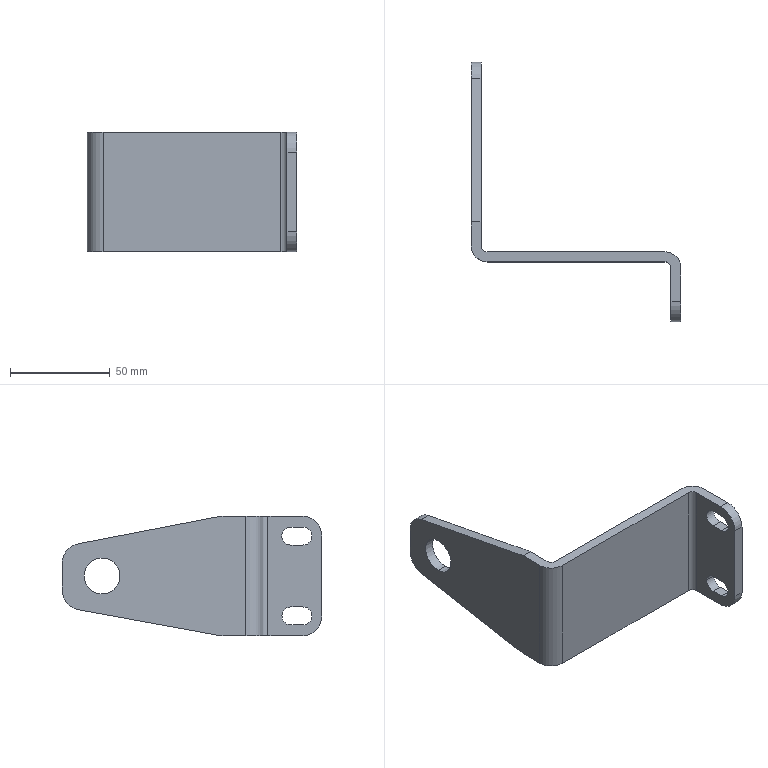Part | SolidWorks | features ICE 4, Fillet 3, Extrusion 1, HoleWzd 1 | 1 solid | 31 faces | box 105 x 130 x 60 mm | volume 58783 mm3 | plane 16 | cylinder 15 | commonest cylinder face diameters 9 x5 20 x4 6 x2 16 x2 18 x2
STEP:
#1=CARTESIAN_POINT('',(0.,-20.,39.));
#2=VERTEX_POINT('',#1);
#3=CARTESIAN_POINT('',(0.,-20.,21.));
#4=VERTEX_POINT('',#3);
#5=CARTESIAN_POINT('',(0.,-20.,30.));
#6=DIRECTION('',(1.,0.,0.));
#7=DIRECTION('',(0.,0.,-1.));
#8=AXIS2_PLACEMENT_3D('',#5,#6,#7);
#9=CIRCLE('',#8,9.);
#10=EDGE_CURVE('',#2,#4,#9,.T.);
#11=ORIENTED_EDGE('',*,*,#10,.T.);
#12=CARTESIAN_POINT('',(-5.,-20.,21.));
#13=VERTEX_POINT('',#12);
#14=CARTESIAN_POINT('',(-5.,-20.,21.));
#15=DIRECTION('',(-1.,0.,0.));
#16=VECTOR('',#15,1000.);
#17=LINE('',#14,#16);
#18=EDGE_CURVE('',#4,#13,#17,.T.);
#19=ORIENTED_EDGE('',*,*,#18,.T.);
#20=CARTESIAN_POINT('',(-5.,-20.,39.));
#21=VERTEX_POINT('',#20);
#22=CARTESIAN_POINT('',(-5.,-20.,30.));
#23=DIRECTION('',(-1.,0.,0.));
#24=DIRECTION('',(0.,0.,1.));
#25=AXIS2_PLACEMENT_3D('',#22,#23,#24);
#26=CIRCLE('',#25,9.);
#27=EDGE_CURVE('',#13,#21,#26,.T.);
#28=ORIENTED_EDGE('',*,*,#27,.T.);
#29=CARTESIAN_POINT('',(-5.,-20.,39.));
#30=DIRECTION('',(-1.,0.,0.));
#31=VECTOR('',#30,1000.);
#32=LINE('',#29,#31);
#33=EDGE_CURVE('',#2,#21,#32,.T.);
#34=ORIENTED_EDGE('',*,*,#33,.F.);
#35=EDGE_LOOP('',(#11,#19,#28,#34));
#36=FACE_OUTER_BOUND('',#35,.T.);
#37=CARTESIAN_POINT('',(-5.,-20.,30.));
#38=DIRECTION('',(-1.,0.,0.));
#39=DIRECTION('',(0.,0.,1.));
#40=AXIS2_PLACEMENT_3D('',#37,#38,#39);
#41=CYLINDRICAL_SURFACE('',#40,9.);
#42=ADVANCED_FACE('',(#36),#41,.F.);
#43=CARTESIAN_POINT('',(95.,-110.,10.));
#44=VERTEX_POINT('',#43);
#45=CARTESIAN_POINT('',(95.,-114.5,14.5));
#46=VERTEX_POINT('',#45);
#47=CARTESIAN_POINT('',(95.,-114.5,10.));
#48=DIRECTION('',(1.,0.,0.));
#49=DIRECTION('',(0.,0.,-1.));
#50=AXIS2_PLACEMENT_3D('',#47,#48,#49);
#51=CIRCLE('',#50,4.5);
#52=EDGE_CURVE('',#44,#46,#51,.T.);
#53=ORIENTED_EDGE('',*,*,#52,.F.);
#54=CARTESIAN_POINT('',(100.,-110.,10.));
#55=VERTEX_POINT('',#54);
#56=CARTESIAN_POINT('',(-5.,-110.,10.));
#57=DIRECTION('',(1.,0.,0.));
#58=VECTOR('',#57,1000.);
#59=LINE('',#56,#58);
#60=EDGE_CURVE('',#44,#55,#59,.T.);
#61=ORIENTED_EDGE('',*,*,#60,.T.);
#62=CARTESIAN_POINT('',(100.,-114.5,14.5));
#63=VERTEX_POINT('',#62);
#64=CARTESIAN_POINT('',(100.,-114.5,10.));
#65=DIRECTION('',(1.,0.,0.));
#66=DIRECTION('',(0.,1.,0.));
#67=AXIS2_PLACEMENT_3D('',#64,#65,#66);
#68=CIRCLE('',#67,4.5);
#69=EDGE_CURVE('',#55,#63,#68,.T.);
#70=ORIENTED_EDGE('',*,*,#69,.T.);
#71=CARTESIAN_POINT('',(-5.,-114.5,14.5));
#72=DIRECTION('',(1.,0.,0.));
#73=VECTOR('',#72,1000.);
#74=LINE('',#71,#73);
#75=EDGE_CURVE('',#46,#63,#74,.T.);
#76=ORIENTED_EDGE('',*,*,#75,.F.);
#77=EDGE_LOOP('',(#53,#61,#70,#76));
#78=FACE_OUTER_BOUND('',#77,.T.);
#79=CARTESIAN_POINT('',(-5.,-114.5,10.));
#80=DIRECTION('',(1.,0.,0.));
#81=DIRECTION('',(0.,1.,0.));
#82=AXIS2_PLACEMENT_3D('',#79,#80,#81);
#83=CYLINDRICAL_SURFACE('',#82,4.5);
#84=ADVANCED_FACE('',(#78),#83,.F.);
#85=CARTESIAN_POINT('',(100.,-120.,0.));
#86=VERTEX_POINT('',#85);
#87=CARTESIAN_POINT('',(100.,-103.,0.));
#88=VERTEX_POINT('',#87);
#89=CARTESIAN_POINT('',(100.,-95.,0.));
#90=DIRECTION('',(0.,1.,0.));
#91=VECTOR('',#90,1000.);
#92=LINE('',#89,#91);
#93=EDGE_CURVE('',#86,#88,#92,.T.);
#94=ORIENTED_EDGE('',*,*,#93,.F.);
#95=CARTESIAN_POINT('',(95.,-120.,0.));
#96=VERTEX_POINT('',#95);
#97=CARTESIAN_POINT('',(-5.,-120.,0.));
#98=DIRECTION('',(-1.,0.,0.));
#99=VECTOR('',#98,1000.);
#100=LINE('',#97,#99);
#101=EDGE_CURVE('',#86,#96,#100,.T.);
#102=ORIENTED_EDGE('',*,*,#101,.T.);
#103=CARTESIAN_POINT('',(95.,-103.,0.));
#104=VERTEX_POINT('',#103);
#105=CARTESIAN_POINT('',(95.,-100.,0.));
#106=DIRECTION('',(0.,-1.,0.));
#107=VECTOR('',#106,1000.);
#108=LINE('',#105,#107);
#109=EDGE_CURVE('',#104,#96,#108,.T.);
#110=ORIENTED_EDGE('',*,*,#109,.F.);
#111=CARTESIAN_POINT('',(92.,-100.,0.));
#112=VERTEX_POINT('',#111);
#113=CARTESIAN_POINT('',(92.,-103.,0.));
#114=DIRECTION('',(0.,0.,1.));
#115=DIRECTION('',(-1.,0.,0.));
#116=AXIS2_PLACEMENT_3D('',#113,#114,#115);
#117=CIRCLE('',#116,3.);
#118=EDGE_CURVE('',#104,#112,#117,.T.);
#119=ORIENTED_EDGE('',*,*,#118,.T.);
#120=CARTESIAN_POINT('',(3.,-100.,0.));
#121=VERTEX_POINT('',#120);
#122=CARTESIAN_POINT('',(-5.,-100.,0.));
#123=DIRECTION('',(1.,0.,0.));
#124=VECTOR('',#123,1000.);
#125=LINE('',#122,#124);
#126=EDGE_CURVE('',#121,#112,#125,.T.);
#127=ORIENTED_EDGE('',*,*,#126,.F.);
#128=CARTESIAN_POINT('',(-5.,-92.,0.));
#129=VERTEX_POINT('',#128);
#130=CARTESIAN_POINT('',(3.,-92.,0.));
#131=DIRECTION('',(0.,0.,-1.));
#132=DIRECTION('',(-1.,0.,0.));
#133=AXIS2_PLACEMENT_3D('',#130,#131,#132);
#134=CIRCLE('',#133,8.);
#135=EDGE_CURVE('',#121,#129,#134,.T.);
#136=ORIENTED_EDGE('',*,*,#135,.T.);
#137=CARTESIAN_POINT('',(-5.,-80.,0.));
#138=VERTEX_POINT('',#137);
#139=CARTESIAN_POINT('',(-5.,-130.,0.));
#140=DIRECTION('',(0.,1.,0.));
#141=VECTOR('',#140,1000.);
#142=LINE('',#139,#141);
#143=EDGE_CURVE('',#129,#138,#142,.T.);
#144=ORIENTED_EDGE('',*,*,#143,.T.);
#145=CARTESIAN_POINT('',(0.,-80.,0.));
#146=VERTEX_POINT('',#145);
#147=CARTESIAN_POINT('',(-5.,-80.,0.));
#148=DIRECTION('',(1.,0.,0.));
#149=VECTOR('',#148,1000.);
#150=LINE('',#147,#149);
#151=EDGE_CURVE('',#138,#146,#150,.T.);
#152=ORIENTED_EDGE('',*,*,#151,.T.);
#153=CARTESIAN_POINT('',(0.,-92.,0.));
#154=VERTEX_POINT('',#153);
#155=CARTESIAN_POINT('',(0.,-130.,0.));
#156=DIRECTION('',(0.,1.,0.));
#157=VECTOR('',#156,1000.);
#158=LINE('',#155,#157);
#159=EDGE_CURVE('',#154,#146,#158,.T.);
#160=ORIENTED_EDGE('',*,*,#159,.F.);
#161=CARTESIAN_POINT('',(3.,-95.,0.));
#162=VERTEX_POINT('',#161);
#163=CARTESIAN_POINT('',(3.,-92.,0.));
#164=DIRECTION('',(0.,0.,1.));
#165=DIRECTION('',(-1.,0.,0.));
#166=AXIS2_PLACEMENT_3D('',#163,#164,#165);
#167=CIRCLE('',#166,3.);
#168=EDGE_CURVE('',#154,#162,#167,.T.);
#169=ORIENTED_EDGE('',*,*,#168,.T.);
#170=CARTESIAN_POINT('',(92.,-95.,0.));
#171=VERTEX_POINT('',#170);
#172=CARTESIAN_POINT('',(100.,-95.,0.));
#173=DIRECTION('',(-1.,0.,0.));
#174=VECTOR('',#173,1000.);
#175=LINE('',#172,#174);
#176=EDGE_CURVE('',#171,#162,#175,.T.);
#177=ORIENTED_EDGE('',*,*,#176,.F.);
#178=CARTESIAN_POINT('',(92.,-103.,0.));
#179=DIRECTION('',(0.,0.,-1.));
#180=DIRECTION('',(-1.,0.,0.));
#181=AXIS2_PLACEMENT_3D('',#178,#179,#180);
#182=CIRCLE('',#181,8.);
#183=EDGE_CURVE('',#171,#88,#182,.T.);
#184=ORIENTED_EDGE('',*,*,#183,.T.);
#185=EDGE_LOOP('',(#94,#102,#110,#119,#127,#136,#144,#152,#160,#169,#177,#184));
#186=FACE_OUTER_BOUND('',#185,.T.);
#187=CARTESIAN_POINT('',(-5.,-130.,0.));
#188=DIRECTION('',(0.,0.,-1.));
#189=DIRECTION('',(-1.,0.,0.));
#190=AXIS2_PLACEMENT_3D('',#187,#188,#189);
#191=PLANE('',#190);
#192=ADVANCED_FACE('',(#186),#191,.T.);
#193=CARTESIAN_POINT('',(100.,-130.,50.));
#194=VERTEX_POINT('',#193);
#195=CARTESIAN_POINT('',(100.,-130.,10.));
#196=VERTEX_POINT('',#195);
#197=CARTESIAN_POINT('',(100.,-130.,0.));
#198=DIRECTION('',(0.,0.,-1.));
#199=VECTOR('',#198,1000.);
#200=LINE('',#197,#199);
#201=EDGE_CURVE('',#194,#196,#200,.T.);
#202=ORIENTED_EDGE('',*,*,#201,.F.);
#203=CARTESIAN_POINT('',(95.,-130.,50.));
#204=VERTEX_POINT('',#203);
#205=CARTESIAN_POINT('',(-5.,-130.,50.));
#206=DIRECTION('',(-1.,0.,0.));
#207=VECTOR('',#206,1000.);
#208=LINE('',#205,#207);
#209=EDGE_CURVE('',#194,#204,#208,.T.);
#210=ORIENTED_EDGE('',*,*,#209,.T.);
#211=CARTESIAN_POINT('',(95.,-130.,10.));
#212=VERTEX_POINT('',#211);
#213=CARTESIAN_POINT('',(95.,-130.,60.));
#214=DIRECTION('',(0.,0.,-1.));
#215=VECTOR('',#214,1000.);
#216=LINE('',#213,#215);
#217=EDGE_CURVE('',#204,#212,#216,.T.);
#218=ORIENTED_EDGE('',*,*,#217,.T.);
#219=CARTESIAN_POINT('',(-5.,-130.,10.));
#220=DIRECTION('',(1.,0.,0.));
#221=VECTOR('',#220,1000.);
#222=LINE('',#219,#221);
#223=EDGE_CURVE('',#212,#196,#222,.T.);
#224=ORIENTED_EDGE('',*,*,#223,.T.);
#225=EDGE_LOOP('',(#202,#210,#218,#224));
#226=FACE_OUTER_BOUND('',#225,.T.);
#227=CARTESIAN_POINT('',(-5.,-130.,60.));
#228=DIRECTION('',(0.,-1.,0.));
#229=DIRECTION('',(0.,0.,-1.));
#230=AXIS2_PLACEMENT_3D('',#227,#228,#229);
#231=PLANE('',#230);
#232=ADVANCED_FACE('',(#226),#231,.T.);
#233=CARTESIAN_POINT('',(95.,-103.,60.));
#234=VERTEX_POINT('',#233);
#235=CARTESIAN_POINT('',(95.,-120.,60.));
#236=VERTEX_POINT('',#235);
#237=CARTESIAN_POINT('',(95.,-100.,60.));
#238=DIRECTION('',(0.,-1.,0.));
#239=VECTOR('',#238,1000.);
#240=LINE('',#237,#239);
#241=EDGE_CURVE('',#234,#236,#240,.T.);
#242=ORIENTED_EDGE('',*,*,#241,.T.);
#243=CARTESIAN_POINT('',(100.,-120.,60.));
#244=VERTEX_POINT('',#243);
#245=CARTESIAN_POINT('',(-5.,-120.,60.));
#246=DIRECTION('',(1.,0.,0.));
#247=VECTOR('',#246,1000.);
#248=LINE('',#245,#247);
#249=EDGE_CURVE('',#236,#244,#248,.T.);
#250=ORIENTED_EDGE('',*,*,#249,.T.);
#251=CARTESIAN_POINT('',(100.,-103.,60.));
#252=VERTEX_POINT('',#251);
#253=CARTESIAN_POINT('',(100.,-130.,60.));
#254=DIRECTION('',(0.,-1.,0.));
#255=VECTOR('',#254,1000.);
#256=LINE('',#253,#255);
#257=EDGE_CURVE('',#252,#244,#256,.T.);
#258=ORIENTED_EDGE('',*,*,#257,.F.);
#259=CARTESIAN_POINT('',(92.,-95.,60.));
#260=VERTEX_POINT('',#259);
#261=CARTESIAN_POINT('',(92.,-103.,60.));
#262=DIRECTION('',(0.,0.,1.));
#263=DIRECTION('',(1.,0.,0.));
#264=AXIS2_PLACEMENT_3D('',#261,#262,#263);
#265=CIRCLE('',#264,8.);
#266=EDGE_CURVE('',#252,#260,#265,.T.);
#267=ORIENTED_EDGE('',*,*,#266,.T.);
#268=CARTESIAN_POINT('',(3.,-95.,60.));
#269=VERTEX_POINT('',#268);
#270=CARTESIAN_POINT('',(100.,-95.,60.));
#271=DIRECTION('',(-1.,0.,0.));
#272=VECTOR('',#271,1000.);
#273=LINE('',#270,#272);
#274=EDGE_CURVE('',#260,#269,#273,.T.);
#275=ORIENTED_EDGE('',*,*,#274,.T.);
#276=CARTESIAN_POINT('',(0.,-92.,60.));
#277=VERTEX_POINT('',#276);
#278=CARTESIAN_POINT('',(3.,-92.,60.));
#279=DIRECTION('',(0.,0.,-1.));
#280=DIRECTION('',(1.,0.,0.));
#281=AXIS2_PLACEMENT_3D('',#278,#279,#280);
#282=CIRCLE('',#281,3.);
#283=EDGE_CURVE('',#269,#277,#282,.T.);
#284=ORIENTED_EDGE('',*,*,#283,.T.);
#285=CARTESIAN_POINT('',(0.,-80.,60.));
#286=VERTEX_POINT('',#285);
#287=CARTESIAN_POINT('',(0.,-80.,60.));
#288=DIRECTION('',(0.,-1.,0.));
#289=VECTOR('',#288,1000.);
#290=LINE('',#287,#289);
#291=EDGE_CURVE('',#286,#277,#290,.T.);
#292=ORIENTED_EDGE('',*,*,#291,.F.);
#293=CARTESIAN_POINT('',(-5.,-80.,60.));
#294=VERTEX_POINT('',#293);
#295=CARTESIAN_POINT('',(-5.,-80.,60.));
#296=DIRECTION('',(1.,0.,0.));
#297=VECTOR('',#296,1000.);
#298=LINE('',#295,#297);
#299=EDGE_CURVE('',#294,#286,#298,.T.);
#300=ORIENTED_EDGE('',*,*,#299,.F.);
#301=CARTESIAN_POINT('',(-5.,-92.,60.));
#302=VERTEX_POINT('',#301);
#303=CARTESIAN_POINT('',(-5.,-80.,60.));
#304=DIRECTION('',(0.,-1.,0.));
#305=VECTOR('',#304,1000.);
#306=LINE('',#303,#305);
#307=EDGE_CURVE('',#294,#302,#306,.T.);
#308=ORIENTED_EDGE('',*,*,#307,.T.);
#309=CARTESIAN_POINT('',(3.,-100.,60.));
#310=VERTEX_POINT('',#309);
#311=CARTESIAN_POINT('',(3.,-92.,60.));
#312=DIRECTION('',(0.,0.,1.));
#313=DIRECTION('',(1.,0.,0.));
#314=AXIS2_PLACEMENT_3D('',#311,#312,#313);
#315=CIRCLE('',#314,8.);
#316=EDGE_CURVE('',#302,#310,#315,.T.);
#317=ORIENTED_EDGE('',*,*,#316,.T.);
#318=CARTESIAN_POINT('',(92.,-100.,60.));
#319=VERTEX_POINT('',#318);
#320=CARTESIAN_POINT('',(-5.,-100.,60.));
#321=DIRECTION('',(1.,0.,0.));
#322=VECTOR('',#321,1000.);
#323=LINE('',#320,#322);
#324=EDGE_CURVE('',#310,#319,#323,.T.);
#325=ORIENTED_EDGE('',*,*,#324,.T.);
#326=CARTESIAN_POINT('',(92.,-103.,60.));
#327=DIRECTION('',(0.,0.,-1.));
#328=DIRECTION('',(1.,0.,0.));
#329=AXIS2_PLACEMENT_3D('',#326,#327,#328);
#330=CIRCLE('',#329,3.);
#331=EDGE_CURVE('',#319,#234,#330,.T.);
#332=ORIENTED_EDGE('',*,*,#331,.T.);
#333=EDGE_LOOP('',(#242,#250,#258,#267,#275,#284,#292,#300,#308,#317,#325,#332));
#334=FACE_OUTER_BOUND('',#333,.T.);
#335=CARTESIAN_POINT('',(-5.,-80.,60.));
#336=DIRECTION('',(0.,0.,1.));
#337=DIRECTION('',(1.,0.,0.));
#338=AXIS2_PLACEMENT_3D('',#335,#336,#337);
#339=PLANE('',#338);
#340=ADVANCED_FACE('',(#334),#339,.T.);
#341=CARTESIAN_POINT('',(0.,-8.11,46.162));
#342=VERTEX_POINT('',#341);
#343=CARTESIAN_POINT('',(0.,0.,44.601));
#344=DIRECTION('',(0.,-0.982,0.189));
#345=VECTOR('',#344,1000.);
#346=LINE('',#343,#345);
#347=EDGE_CURVE('',#342,#286,#346,.T.);
#348=ORIENTED_EDGE('',*,*,#347,.F.);
#349=CARTESIAN_POINT('',(-5.,-8.11,46.162));
#350=VERTEX_POINT('',#349);
#351=CARTESIAN_POINT('',(-5.,-8.11,46.162));
#352=DIRECTION('',(-1.,0.,0.));
#353=VECTOR('',#352,1000.);
#354=LINE('',#351,#353);
#355=EDGE_CURVE('',#342,#350,#354,.T.);
#356=ORIENTED_EDGE('',*,*,#355,.T.);
#357=CARTESIAN_POINT('',(-5.,0.,44.601));
#358=DIRECTION('',(0.,-0.982,0.189));
#359=VECTOR('',#358,1000.);
#360=LINE('',#357,#359);
#361=EDGE_CURVE('',#350,#294,#360,.T.);
#362=ORIENTED_EDGE('',*,*,#361,.T.);
#363=ORIENTED_EDGE('',*,*,#299,.T.);
#364=EDGE_LOOP('',(#348,#356,#362,#363));
#365=FACE_OUTER_BOUND('',#364,.T.);
#366=CARTESIAN_POINT('',(-5.,0.,44.601));
#367=DIRECTION('',(0.,0.189,0.982));
#368=DIRECTION('',(0.,-0.982,0.189));
#369=AXIS2_PLACEMENT_3D('',#366,#367,#368);
#370=PLANE('',#369);
#371=ADVANCED_FACE('',(#365),#370,.T.);
#372=CARTESIAN_POINT('',(0.,0.,22.941));
#373=VERTEX_POINT('',#372);
#374=CARTESIAN_POINT('',(0.,0.,36.342));
#375=VERTEX_POINT('',#374);
#376=CARTESIAN_POINT('',(0.,0.,14.601));
#377=DIRECTION('',(0.,0.,1.));
#378=VECTOR('',#377,1000.);
#379=LINE('',#376,#378);
#380=EDGE_CURVE('',#373,#375,#379,.T.);
#381=ORIENTED_EDGE('',*,*,#380,.F.);
#382=CARTESIAN_POINT('',(-5.,0.,22.941));
#383=VERTEX_POINT('',#382);
#384=CARTESIAN_POINT('',(-5.,0.,22.941));
#385=DIRECTION('',(-1.,0.,0.));
#386=VECTOR('',#385,1000.);
#387=LINE('',#384,#386);
#388=EDGE_CURVE('',#373,#383,#387,.T.);
#389=ORIENTED_EDGE('',*,*,#388,.T.);
#390=CARTESIAN_POINT('',(-5.,0.,36.342));
#391=VERTEX_POINT('',#390);
#392=CARTESIAN_POINT('',(-5.,0.,14.601));
#393=DIRECTION('',(0.,0.,1.));
#394=VECTOR('',#393,1000.);
#395=LINE('',#392,#394);
#396=EDGE_CURVE('',#383,#391,#395,.T.);
#397=ORIENTED_EDGE('',*,*,#396,.T.);
#398=CARTESIAN_POINT('',(-5.,0.,36.342));
#399=DIRECTION('',(1.,0.,0.));
#400=VECTOR('',#399,1000.);
#401=LINE('',#398,#400);
#402=EDGE_CURVE('',#391,#375,#401,.T.);
#403=ORIENTED_EDGE('',*,*,#402,.T.);
#404=EDGE_LOOP('',(#381,#389,#397,#403));
#405=FACE_OUTER_BOUND('',#404,.T.);
#406=CARTESIAN_POINT('',(-5.,0.,14.601));
#407=DIRECTION('',(0.,1.,0.));
#408=DIRECTION('',(0.,0.,1.));
#409=AXIS2_PLACEMENT_3D('',#406,#407,#408);
#410=PLANE('',#409);
#411=ADVANCED_FACE('',(#405),#410,.T.);
#412=CARTESIAN_POINT('',(-5.,-8.205,13.103));
#413=VERTEX_POINT('',#412);
#414=CARTESIAN_POINT('',(-5.,-80.,0.));
#415=DIRECTION('',(0.,0.9838,0.1795));
#416=VECTOR('',#415,1000.);
#417=LINE('',#414,#416);
#418=EDGE_CURVE('',#138,#413,#417,.T.);
#419=ORIENTED_EDGE('',*,*,#418,.T.);
#420=CARTESIAN_POINT('',(0.,-8.205,13.103));
#421=VERTEX_POINT('',#420);
#422=CARTESIAN_POINT('',(-5.,-8.205,13.103));
#423=DIRECTION('',(1.,0.,0.));
#424=VECTOR('',#423,1000.);
#425=LINE('',#422,#424);
#426=EDGE_CURVE('',#413,#421,#425,.T.);
#427=ORIENTED_EDGE('',*,*,#426,.T.);
#428=CARTESIAN_POINT('',(0.,-80.,0.));
#429=DIRECTION('',(0.,0.9838,0.1795));
#430=VECTOR('',#429,1000.);
#431=LINE('',#428,#430);
#432=EDGE_CURVE('',#146,#421,#431,.T.);
#433=ORIENTED_EDGE('',*,*,#432,.F.);
#434=ORIENTED_EDGE('',*,*,#151,.F.);
#435=EDGE_LOOP('',(#419,#427,#433,#434));
#436=FACE_OUTER_BOUND('',#435,.T.);
#437=CARTESIAN_POINT('',(-5.,-80.,0.));
#438=DIRECTION('',(0.,0.1795,-0.9838));
#439=DIRECTION('',(0.,0.9838,0.1795));
#440=AXIS2_PLACEMENT_3D('',#437,#438,#439);
#441=PLANE('',#440);
#442=ADVANCED_FACE('',(#436),#441,.T.);
#443=CARTESIAN_POINT('',(-5.,-20.,30.));
#444=DIRECTION('',(-1.,0.,0.));
#445=DIRECTION('',(0.,0.,1.));
#446=AXIS2_PLACEMENT_3D('',#443,#444,#445);
#447=CIRCLE('',#446,9.);
#448=EDGE_CURVE('',#21,#13,#447,.T.);
#449=ORIENTED_EDGE('',*,*,#448,.F.);
#450=ORIENTED_EDGE('',*,*,#27,.F.);
#451=EDGE_LOOP('',(#449,#450));
#452=FACE_BOUND('',#451,.T.);
#453=ORIENTED_EDGE('',*,*,#396,.F.);
#454=CARTESIAN_POINT('',(-5.,-10.,22.941));
#455=DIRECTION('',(-1.,0.,0.));
#456=DIRECTION('',(0.,0.,-1.));
#457=AXIS2_PLACEMENT_3D('',#454,#455,#456);
#458=CIRCLE('',#457,10.);
#459=EDGE_CURVE('',#383,#413,#458,.T.);
#460=ORIENTED_EDGE('',*,*,#459,.T.);
#461=ORIENTED_EDGE('',*,*,#418,.F.);
#462=ORIENTED_EDGE('',*,*,#143,.F.);
#463=CARTESIAN_POINT('',(-5.,-92.,0.));
#464=DIRECTION('',(0.,0.,1.));
#465=VECTOR('',#464,1000.);
#466=LINE('',#463,#465);
#467=EDGE_CURVE('',#129,#302,#466,.T.);
#468=ORIENTED_EDGE('',*,*,#467,.T.);
#469=ORIENTED_EDGE('',*,*,#307,.F.);
#470=ORIENTED_EDGE('',*,*,#361,.F.);
#471=CARTESIAN_POINT('',(-5.,-10.,36.342));
#472=DIRECTION('',(-1.,0.,0.));
#473=DIRECTION('',(0.,0.,-1.));
#474=AXIS2_PLACEMENT_3D('',#471,#472,#473);
#475=CIRCLE('',#474,10.);
#476=EDGE_CURVE('',#350,#391,#475,.T.);
#477=ORIENTED_EDGE('',*,*,#476,.T.);
#478=EDGE_LOOP('',(#453,#460,#461,#462,#468,#469,#470,#477));
#479=FACE_OUTER_BOUND('',#478,.T.);
#480=CARTESIAN_POINT('',(-5.,0.,0.));
#481=DIRECTION('',(1.,0.,0.));
#482=DIRECTION('',(0.,0.,-1.));
#483=AXIS2_PLACEMENT_3D('',#480,#481,#482);
#484=PLANE('',#483);
#485=ADVANCED_FACE('',(#452,#479),#484,.F.);
#486=ORIENTED_EDGE('',*,*,#10,.F.);
#487=CARTESIAN_POINT('',(0.,-20.,30.));
#488=DIRECTION('',(1.,0.,0.));
#489=DIRECTION('',(0.,0.,-1.));
#490=AXIS2_PLACEMENT_3D('',#487,#488,#489);
#491=CIRCLE('',#490,9.);
#492=EDGE_CURVE('',#4,#2,#491,.T.);
#493=ORIENTED_EDGE('',*,*,#492,.F.);
#494=EDGE_LOOP('',(#486,#493));
#495=FACE_BOUND('',#494,.T.);
#496=ORIENTED_EDGE('',*,*,#432,.T.);
#497=CARTESIAN_POINT('',(0.,-10.,22.941));
#498=DIRECTION('',(1.,0.,0.));
#499=DIRECTION('',(0.,0.,-1.));
#500=AXIS2_PLACEMENT_3D('',#497,#498,#499);
#501=CIRCLE('',#500,10.);
#502=EDGE_CURVE('',#421,#373,#501,.T.);
#503=ORIENTED_EDGE('',*,*,#502,.T.);
#504=ORIENTED_EDGE('',*,*,#380,.T.);
#505=CARTESIAN_POINT('',(0.,-10.,36.342));
#506=DIRECTION('',(1.,0.,0.));
#507=DIRECTION('',(0.,0.,-1.));
#508=AXIS2_PLACEMENT_3D('',#505,#506,#507);
#509=CIRCLE('',#508,10.);
#510=EDGE_CURVE('',#375,#342,#509,.T.);
#511=ORIENTED_EDGE('',*,*,#510,.T.);
#512=ORIENTED_EDGE('',*,*,#347,.T.);
#513=ORIENTED_EDGE('',*,*,#291,.T.);
#514=CARTESIAN_POINT('',(0.,-92.,0.));
#515=DIRECTION('',(0.,0.,-1.));
#516=VECTOR('',#515,1000.);
#517=LINE('',#514,#516);
#518=EDGE_CURVE('',#277,#154,#517,.T.);
#519=ORIENTED_EDGE('',*,*,#518,.T.);
#520=ORIENTED_EDGE('',*,*,#159,.T.);
#521=EDGE_LOOP('',(#496,#503,#504,#511,#512,#513,#519,#520));
#522=FACE_OUTER_BOUND('',#521,.T.);
#523=CARTESIAN_POINT('',(0.,0.,0.));
#524=DIRECTION('',(1.,0.,0.));
#525=DIRECTION('',(0.,0.,-1.));
#526=AXIS2_PLACEMENT_3D('',#523,#524,#525);
#527=PLANE('',#526);
#528=ADVANCED_FACE('',(#495,#522),#527,.T.);
#529=ORIENTED_EDGE('',*,*,#274,.F.);
#530=CARTESIAN_POINT('',(92.,-95.,60.));
#531=DIRECTION('',(0.,0.,-1.));
#532=VECTOR('',#531,1000.);
#533=LINE('',#530,#532);
#534=EDGE_CURVE('',#260,#171,#533,.T.);
#535=ORIENTED_EDGE('',*,*,#534,.T.);
#536=ORIENTED_EDGE('',*,*,#176,.T.);
#537=CARTESIAN_POINT('',(3.,-95.,60.));
#538=DIRECTION('',(0.,0.,1.));
#539=VECTOR('',#538,1000.);
#540=LINE('',#537,#539);
#541=EDGE_CURVE('',#162,#269,#540,.T.);
#542=ORIENTED_EDGE('',*,*,#541,.T.);
#543=EDGE_LOOP('',(#529,#535,#536,#542));
#544=FACE_OUTER_BOUND('',#543,.T.);
#545=CARTESIAN_POINT('',(100.,-95.,60.));
#546=DIRECTION('',(0.,-1.,0.));
#547=DIRECTION('',(1.,0.,0.));
#548=AXIS2_PLACEMENT_3D('',#545,#546,#547);
#549=PLANE('',#548);
#550=ADVANCED_FACE('',(#544),#549,.F.);
#551=CARTESIAN_POINT('',(100.,-120.5,14.5));
#552=VERTEX_POINT('',#551);
#553=CARTESIAN_POINT('',(100.,-114.5,14.5));
#554=DIRECTION('',(0.,-1.,0.));
#555=VECTOR('',#554,1000.);
#556=LINE('',#553,#555);
#557=EDGE_CURVE('',#63,#552,#556,.T.);
#558=ORIENTED_EDGE('',*,*,#557,.F.);
#559=ORIENTED_EDGE('',*,*,#69,.F.);
#560=CARTESIAN_POINT('',(100.,-114.5,5.5));
#561=VERTEX_POINT('',#560);
#562=CARTESIAN_POINT('',(100.,-114.5,10.));
#563=DIRECTION('',(1.,0.,0.));
#564=DIRECTION('',(0.,1.,0.));
#565=AXIS2_PLACEMENT_3D('',#562,#563,#564);
#566=CIRCLE('',#565,4.5);
#567=EDGE_CURVE('',#561,#55,#566,.T.);
#568=ORIENTED_EDGE('',*,*,#567,.F.);
#569=CARTESIAN_POINT('',(100.,-120.5,5.5));
#570=VERTEX_POINT('',#569);
#571=CARTESIAN_POINT('',(100.,-120.5,5.5));
#572=DIRECTION('',(0.,1.,0.));
#573=VECTOR('',#572,1000.);
#574=LINE('',#571,#573);
#575=EDGE_CURVE('',#570,#561,#574,.T.);
#576=ORIENTED_EDGE('',*,*,#575,.F.);
#577=CARTESIAN_POINT('',(100.,-120.5,10.));
#578=DIRECTION('',(1.,0.,0.));
#579=DIRECTION('',(0.,1.,0.));
#580=AXIS2_PLACEMENT_3D('',#577,#578,#579);
#581=CIRCLE('',#580,4.5);
#582=EDGE_CURVE('',#552,#570,#581,.T.);
#583=ORIENTED_EDGE('',*,*,#582,.F.);
#584=EDGE_LOOP('',(#558,#559,#568,#576,#583));
#585=FACE_BOUND('',#584,.T.);
#586=CARTESIAN_POINT('',(100.,-114.5,45.5));
#587=VERTEX_POINT('',#586);
#588=CARTESIAN_POINT('',(100.,-120.5,45.5));
#589=VERTEX_POINT('',#588);
#590=CARTESIAN_POINT('',(100.,-114.5,45.5));
#591=DIRECTION('',(0.,-1.,0.));
#592=VECTOR('',#591,1000.);
#593=LINE('',#590,#592);
#594=EDGE_CURVE('',#587,#589,#593,.T.);
#595=ORIENTED_EDGE('',*,*,#594,.T.);
#596=CARTESIAN_POINT('',(100.,-120.5,54.5));
#597=VERTEX_POINT('',#596);
#598=CARTESIAN_POINT('',(100.,-120.5,50.));
#599=DIRECTION('',(-1.,0.,0.));
#600=DIRECTION('',(0.,0.,1.));
#601=AXIS2_PLACEMENT_3D('',#598,#599,#600);
#602=CIRCLE('',#601,4.5);
#603=EDGE_CURVE('',#589,#597,#602,.T.);
#604=ORIENTED_EDGE('',*,*,#603,.T.);
#605=CARTESIAN_POINT('',(100.,-114.5,54.5));
#606=VERTEX_POINT('',#605);
#607=CARTESIAN_POINT('',(100.,-120.5,54.5));
#608=DIRECTION('',(0.,1.,0.));
#609=VECTOR('',#608,1000.);
#610=LINE('',#607,#609);
#611=EDGE_CURVE('',#597,#606,#610,.T.);
#612=ORIENTED_EDGE('',*,*,#611,.T.);
#613=CARTESIAN_POINT('',(100.,-114.5,50.));
#614=DIRECTION('',(-1.,0.,0.));
#615=DIRECTION('',(0.,0.,1.));
#616=AXIS2_PLACEMENT_3D('',#613,#614,#615);
#617=CIRCLE('',#616,4.5);
#618=EDGE_CURVE('',#606,#587,#617,.T.);
#619=ORIENTED_EDGE('',*,*,#618,.T.);
#620=EDGE_LOOP('',(#595,#604,#612,#619));
#621=FACE_BOUND('',#620,.T.);
#622=ORIENTED_EDGE('',*,*,#257,.T.);
#623=CARTESIAN_POINT('',(100.,-120.,50.));
#624=DIRECTION('',(1.,0.,0.));
#625=DIRECTION('',(0.,-1.,0.));
#626=AXIS2_PLACEMENT_3D('',#623,#624,#625);
#627=CIRCLE('',#626,10.);
#628=EDGE_CURVE('',#244,#194,#627,.T.);
#629=ORIENTED_EDGE('',*,*,#628,.T.);
#630=ORIENTED_EDGE('',*,*,#201,.T.);
#631=CARTESIAN_POINT('',(100.,-120.,10.));
#632=DIRECTION('',(1.,0.,0.));
#633=DIRECTION('',(0.,-1.,0.));
#634=AXIS2_PLACEMENT_3D('',#631,#632,#633);
#635=CIRCLE('',#634,10.);
#636=EDGE_CURVE('',#196,#86,#635,.T.);
#637=ORIENTED_EDGE('',*,*,#636,.T.);
#638=ORIENTED_EDGE('',*,*,#93,.T.);
#639=CARTESIAN_POINT('',(100.,-103.,0.));
#640=DIRECTION('',(0.,0.,1.));
#641=VECTOR('',#640,1000.);
#642=LINE('',#639,#641);
#643=EDGE_CURVE('',#88,#252,#642,.T.);
#644=ORIENTED_EDGE('',*,*,#643,.T.);
#645=EDGE_LOOP('',(#622,#629,#630,#637,#638,#644));
#646=FACE_OUTER_BOUND('',#645,.T.);
#647=CARTESIAN_POINT('',(100.,0.,0.));
#648=DIRECTION('',(-1.,0.,0.));
#649=DIRECTION('',(0.,-1.,0.));
#650=AXIS2_PLACEMENT_3D('',#647,#648,#649);
#651=PLANE('',#650);
#652=ADVANCED_FACE('',(#585,#621,#646),#651,.F.);
#653=ORIENTED_EDGE('',*,*,#324,.F.);
#654=CARTESIAN_POINT('',(3.,-100.,60.));
#655=DIRECTION('',(0.,0.,-1.));
#656=VECTOR('',#655,1000.);
#657=LINE('',#654,#656);
#658=EDGE_CURVE('',#310,#121,#657,.T.);
#659=ORIENTED_EDGE('',*,*,#658,.T.);
#660=ORIENTED_EDGE('',*,*,#126,.T.);
#661=CARTESIAN_POINT('',(92.,-100.,60.));
#662=DIRECTION('',(0.,0.,1.));
#663=VECTOR('',#662,1000.);
#664=LINE('',#661,#663);
#665=EDGE_CURVE('',#112,#319,#664,.T.);
#666=ORIENTED_EDGE('',*,*,#665,.T.);
#667=EDGE_LOOP('',(#653,#659,#660,#666));
#668=FACE_OUTER_BOUND('',#667,.T.);
#669=CARTESIAN_POINT('',(-5.,-100.,60.));
#670=DIRECTION('',(0.,1.,0.));
#671=DIRECTION('',(0.,0.,1.));
#672=AXIS2_PLACEMENT_3D('',#669,#670,#671);
#673=PLANE('',#672);
#674=ADVANCED_FACE('',(#668),#673,.F.);
#675=CARTESIAN_POINT('',(95.,-120.5,5.5));
#676=VERTEX_POINT('',#675);
#677=CARTESIAN_POINT('',(95.,-114.5,5.5));
#678=VERTEX_POINT('',#677);
#679=CARTESIAN_POINT('',(95.,-100.,5.5));
#680=DIRECTION('',(0.,1.,0.));
#681=VECTOR('',#680,1000.);
#682=LINE('',#679,#681);
#683=EDGE_CURVE('',#676,#678,#682,.T.);
#684=ORIENTED_EDGE('',*,*,#683,.T.);
#685=CARTESIAN_POINT('',(95.,-114.5,10.));
#686=DIRECTION('',(1.,0.,0.));
#687=DIRECTION('',(0.,0.,-1.));
#688=AXIS2_PLACEMENT_3D('',#685,#686,#687);
#689=CIRCLE('',#688,4.5);
#690=EDGE_CURVE('',#678,#44,#689,.T.);
#691=ORIENTED_EDGE('',*,*,#690,.T.);
#692=ORIENTED_EDGE('',*,*,#52,.T.);
#693=CARTESIAN_POINT('',(95.,-120.5,14.5));
#694=VERTEX_POINT('',#693);
#695=CARTESIAN_POINT('',(95.,-100.,14.5));
#696=DIRECTION('',(0.,-1.,0.));
#697=VECTOR('',#696,1000.);
#698=LINE('',#695,#697);
#699=EDGE_CURVE('',#46,#694,#698,.T.);
#700=ORIENTED_EDGE('',*,*,#699,.T.);
#701=CARTESIAN_POINT('',(95.,-120.5,10.));
#702=DIRECTION('',(1.,0.,0.));
#703=DIRECTION('',(0.,0.,-1.));
#704=AXIS2_PLACEMENT_3D('',#701,#702,#703);
#705=CIRCLE('',#704,4.5);
#706=EDGE_CURVE('',#694,#676,#705,.T.);
#707=ORIENTED_EDGE('',*,*,#706,.T.);
#708=EDGE_LOOP('',(#684,#691,#692,#700,#707));
#709=FACE_BOUND('',#708,.T.);
#710=CARTESIAN_POINT('',(95.,-120.5,54.5));
#711=VERTEX_POINT('',#710);
#712=CARTESIAN_POINT('',(95.,-114.5,54.5));
#713=VERTEX_POINT('',#712);
#714=CARTESIAN_POINT('',(95.,-120.5,54.5));
#715=DIRECTION('',(0.,1.,0.));
#716=VECTOR('',#715,1000.);
#717=LINE('',#714,#716);
#718=EDGE_CURVE('',#711,#713,#717,.T.);
#719=ORIENTED_EDGE('',*,*,#718,.F.);
#720=CARTESIAN_POINT('',(95.,-120.5,45.5));
#721=VERTEX_POINT('',#720);
#722=CARTESIAN_POINT('',(95.,-120.5,50.));
#723=DIRECTION('',(-1.,0.,0.));
#724=DIRECTION('',(0.,0.,1.));
#725=AXIS2_PLACEMENT_3D('',#722,#723,#724);
#726=CIRCLE('',#725,4.5);
#727=EDGE_CURVE('',#721,#711,#726,.T.);
#728=ORIENTED_EDGE('',*,*,#727,.F.);
#729=CARTESIAN_POINT('',(95.,-114.5,45.5));
#730=VERTEX_POINT('',#729);
#731=CARTESIAN_POINT('',(95.,-114.5,45.5));
#732=DIRECTION('',(0.,-1.,0.));
#733=VECTOR('',#732,1000.);
#734=LINE('',#731,#733);
#735=EDGE_CURVE('',#730,#721,#734,.T.);
#736=ORIENTED_EDGE('',*,*,#735,.F.);
#737=CARTESIAN_POINT('',(95.,-114.5,50.));
#738=DIRECTION('',(-1.,0.,0.));
#739=DIRECTION('',(0.,0.,1.));
#740=AXIS2_PLACEMENT_3D('',#737,#738,#739);
#741=CIRCLE('',#740,4.5);
#742=EDGE_CURVE('',#713,#730,#741,.T.);
#743=ORIENTED_EDGE('',*,*,#742,.F.);
#744=EDGE_LOOP('',(#719,#728,#736,#743));
#745=FACE_BOUND('',#744,.T.);
#746=ORIENTED_EDGE('',*,*,#217,.F.);
#747=CARTESIAN_POINT('',(95.,-120.,50.));
#748=DIRECTION('',(-1.,0.,0.));
#749=DIRECTION('',(0.,0.,-1.));
#750=AXIS2_PLACEMENT_3D('',#747,#748,#749);
#751=CIRCLE('',#750,10.);
#752=EDGE_CURVE('',#204,#236,#751,.T.);
#753=ORIENTED_EDGE('',*,*,#752,.T.);
#754=ORIENTED_EDGE('',*,*,#241,.F.);
#755=CARTESIAN_POINT('',(95.,-103.,0.));
#756=DIRECTION('',(0.,0.,-1.));
#757=VECTOR('',#756,1000.);
#758=LINE('',#755,#757);
#759=EDGE_CURVE('',#234,#104,#758,.T.);
#760=ORIENTED_EDGE('',*,*,#759,.T.);
#761=ORIENTED_EDGE('',*,*,#109,.T.);
#762=CARTESIAN_POINT('',(95.,-120.,10.));
#763=DIRECTION('',(-1.,0.,0.));
#764=DIRECTION('',(0.,0.,-1.));
#765=AXIS2_PLACEMENT_3D('',#762,#763,#764);
#766=CIRCLE('',#765,10.);
#767=EDGE_CURVE('',#96,#212,#766,.T.);
#768=ORIENTED_EDGE('',*,*,#767,.T.);
#769=EDGE_LOOP('',(#746,#753,#754,#760,#761,#768));
#770=FACE_OUTER_BOUND('',#769,.T.);
#771=CARTESIAN_POINT('',(95.,-100.,60.));
#772=DIRECTION('',(1.,0.,0.));
#773=DIRECTION('',(0.,0.,-1.));
#774=AXIS2_PLACEMENT_3D('',#771,#772,#773);
#775=PLANE('',#774);
#776=ADVANCED_FACE('',(#709,#745,#770),#775,.F.);
#777=ORIENTED_EDGE('',*,*,#727,.T.);
#778=CARTESIAN_POINT('',(100.,-120.5,54.5));
#779=DIRECTION('',(-1.,0.,0.));
#780=VECTOR('',#779,1000.);
#781=LINE('',#778,#780);
#782=EDGE_CURVE('',#597,#711,#781,.T.);
#783=ORIENTED_EDGE('',*,*,#782,.F.);
#784=ORIENTED_EDGE('',*,*,#603,.F.);
#785=CARTESIAN_POINT('',(100.,-120.5,45.5));
#786=DIRECTION('',(-1.,0.,0.));
#787=VECTOR('',#786,1000.);
#788=LINE('',#785,#787);
#789=EDGE_CURVE('',#589,#721,#788,.T.);
#790=ORIENTED_EDGE('',*,*,#789,.T.);
#791=EDGE_LOOP('',(#777,#783,#784,#790));
#792=FACE_OUTER_BOUND('',#791,.T.);
#793=CARTESIAN_POINT('',(100.,-120.5,50.));
#794=DIRECTION('',(-1.,0.,0.));
#795=DIRECTION('',(0.,0.,1.));
#796=AXIS2_PLACEMENT_3D('',#793,#794,#795);
#797=CYLINDRICAL_SURFACE('',#796,4.5);
#798=ADVANCED_FACE('',(#792),#797,.F.);
#799=ORIENTED_EDGE('',*,*,#735,.T.);
#800=ORIENTED_EDGE('',*,*,#789,.F.);
#801=ORIENTED_EDGE('',*,*,#594,.F.);
#802=CARTESIAN_POINT('',(100.,-114.5,45.5));
#803=DIRECTION('',(-1.,0.,0.));
#804=VECTOR('',#803,1000.);
#805=LINE('',#802,#804);
#806=EDGE_CURVE('',#587,#730,#805,.T.);
#807=ORIENTED_EDGE('',*,*,#806,.T.);
#808=EDGE_LOOP('',(#799,#800,#801,#807));
#809=FACE_OUTER_BOUND('',#808,.T.);
#810=CARTESIAN_POINT('',(100.,-114.5,45.5));
#811=DIRECTION('',(0.,0.,-1.));
#812=DIRECTION('',(-1.,0.,0.));
#813=AXIS2_PLACEMENT_3D('',#810,#811,#812);
#814=PLANE('',#813);
#815=ADVANCED_FACE('',(#809),#814,.F.);
#816=ORIENTED_EDGE('',*,*,#742,.T.);
#817=ORIENTED_EDGE('',*,*,#806,.F.);
#818=ORIENTED_EDGE('',*,*,#618,.F.);
#819=CARTESIAN_POINT('',(100.,-114.5,54.5));
#820=DIRECTION('',(-1.,0.,0.));
#821=VECTOR('',#820,1000.);
#822=LINE('',#819,#821);
#823=EDGE_CURVE('',#606,#713,#822,.T.);
#824=ORIENTED_EDGE('',*,*,#823,.T.);
#825=EDGE_LOOP('',(#816,#817,#818,#824));
#826=FACE_OUTER_BOUND('',#825,.T.);
#827=CARTESIAN_POINT('',(100.,-114.5,50.));
#828=DIRECTION('',(-1.,0.,0.));
#829=DIRECTION('',(0.,0.,1.));
#830=AXIS2_PLACEMENT_3D('',#827,#828,#829);
#831=CYLINDRICAL_SURFACE('',#830,4.5);
#832=ADVANCED_FACE('',(#826),#831,.F.);
#833=ORIENTED_EDGE('',*,*,#718,.T.);
#834=ORIENTED_EDGE('',*,*,#823,.F.);
#835=ORIENTED_EDGE('',*,*,#611,.F.);
#836=ORIENTED_EDGE('',*,*,#782,.T.);
#837=EDGE_LOOP('',(#833,#834,#835,#836));
#838=FACE_OUTER_BOUND('',#837,.T.);
#839=CARTESIAN_POINT('',(100.,-120.5,54.5));
#840=DIRECTION('',(0.,0.,1.));
#841=DIRECTION('',(1.,0.,0.));
#842=AXIS2_PLACEMENT_3D('',#839,#840,#841);
#843=PLANE('',#842);
#844=ADVANCED_FACE('',(#838),#843,.F.);
#845=ORIENTED_EDGE('',*,*,#60,.F.);
#846=ORIENTED_EDGE('',*,*,#690,.F.);
#847=CARTESIAN_POINT('',(-5.,-114.5,5.5));
#848=DIRECTION('',(1.,0.,0.));
#849=VECTOR('',#848,1000.);
#850=LINE('',#847,#849);
#851=EDGE_CURVE('',#678,#561,#850,.T.);
#852=ORIENTED_EDGE('',*,*,#851,.T.);
#853=ORIENTED_EDGE('',*,*,#567,.T.);
#854=EDGE_LOOP('',(#845,#846,#852,#853));
#855=FACE_OUTER_BOUND('',#854,.T.);
#856=CARTESIAN_POINT('',(-5.,-114.5,10.));
#857=DIRECTION('',(1.,0.,0.));
#858=DIRECTION('',(0.,1.,0.));
#859=AXIS2_PLACEMENT_3D('',#856,#857,#858);
#860=CYLINDRICAL_SURFACE('',#859,4.5);
#861=ADVANCED_FACE('',(#855),#860,.F.);
#862=CARTESIAN_POINT('',(-5.,-120.5,5.5));
#863=DIRECTION('',(1.,0.,0.));
#864=VECTOR('',#863,1000.);
#865=LINE('',#862,#864);
#866=EDGE_CURVE('',#676,#570,#865,.T.);
#867=ORIENTED_EDGE('',*,*,#866,.T.);
#868=ORIENTED_EDGE('',*,*,#575,.T.);
#869=ORIENTED_EDGE('',*,*,#851,.F.);
#870=ORIENTED_EDGE('',*,*,#683,.F.);
#871=EDGE_LOOP('',(#867,#868,#869,#870));
#872=FACE_OUTER_BOUND('',#871,.T.);
#873=CARTESIAN_POINT('',(-5.,-120.5,5.5));
#874=DIRECTION('',(0.,0.,-1.));
#875=DIRECTION('',(-1.,0.,0.));
#876=AXIS2_PLACEMENT_3D('',#873,#874,#875);
#877=PLANE('',#876);
#878=ADVANCED_FACE('',(#872),#877,.F.);
#879=CARTESIAN_POINT('',(-5.,-120.5,14.5));
#880=DIRECTION('',(1.,0.,0.));
#881=VECTOR('',#880,1000.);
#882=LINE('',#879,#881);
#883=EDGE_CURVE('',#694,#552,#882,.T.);
#884=ORIENTED_EDGE('',*,*,#883,.T.);
#885=ORIENTED_EDGE('',*,*,#582,.T.);
#886=ORIENTED_EDGE('',*,*,#866,.F.);
#887=ORIENTED_EDGE('',*,*,#706,.F.);
#888=EDGE_LOOP('',(#884,#885,#886,#887));
#889=FACE_OUTER_BOUND('',#888,.T.);
#890=CARTESIAN_POINT('',(-5.,-120.5,10.));
#891=DIRECTION('',(1.,0.,0.));
#892=DIRECTION('',(0.,1.,0.));
#893=AXIS2_PLACEMENT_3D('',#890,#891,#892);
#894=CYLINDRICAL_SURFACE('',#893,4.5);
#895=ADVANCED_FACE('',(#889),#894,.F.);
#896=ORIENTED_EDGE('',*,*,#75,.T.);
#897=ORIENTED_EDGE('',*,*,#557,.T.);
#898=ORIENTED_EDGE('',*,*,#883,.F.);
#899=ORIENTED_EDGE('',*,*,#699,.F.);
#900=EDGE_LOOP('',(#896,#897,#898,#899));
#901=FACE_OUTER_BOUND('',#900,.T.);
#902=CARTESIAN_POINT('',(-5.,-114.5,14.5));
#903=DIRECTION('',(0.,0.,1.));
#904=DIRECTION('',(0.,-1.,0.));
#905=AXIS2_PLACEMENT_3D('',#902,#903,#904);
#906=PLANE('',#905);
#907=ADVANCED_FACE('',(#901),#906,.F.);
#908=ORIENTED_EDGE('',*,*,#18,.F.);
#909=ORIENTED_EDGE('',*,*,#492,.T.);
#910=ORIENTED_EDGE('',*,*,#33,.T.);
#911=ORIENTED_EDGE('',*,*,#448,.T.);
#912=EDGE_LOOP('',(#908,#909,#910,#911));
#913=FACE_OUTER_BOUND('',#912,.T.);
#914=CARTESIAN_POINT('',(-5.,-20.,30.));
#915=DIRECTION('',(-1.,0.,0.));
#916=DIRECTION('',(0.,0.,1.));
#917=AXIS2_PLACEMENT_3D('',#914,#915,#916);
#918=CYLINDRICAL_SURFACE('',#917,9.);
#919=ADVANCED_FACE('',(#913),#918,.F.);
#920=ORIENTED_EDGE('',*,*,#168,.F.);
#921=ORIENTED_EDGE('',*,*,#518,.F.);
#922=ORIENTED_EDGE('',*,*,#283,.F.);
#923=ORIENTED_EDGE('',*,*,#541,.F.);
#924=EDGE_LOOP('',(#920,#921,#922,#923));
#925=FACE_OUTER_BOUND('',#924,.T.);
#926=CARTESIAN_POINT('',(3.,-92.,60.));
#927=DIRECTION('',(0.,0.,1.));
#928=DIRECTION('',(0.,-1.,0.));
#929=AXIS2_PLACEMENT_3D('',#926,#927,#928);
#930=CYLINDRICAL_SURFACE('',#929,3.);
#931=ADVANCED_FACE('',(#925),#930,.F.);
#932=ORIENTED_EDGE('',*,*,#331,.F.);
#933=ORIENTED_EDGE('',*,*,#665,.F.);
#934=ORIENTED_EDGE('',*,*,#118,.F.);
#935=ORIENTED_EDGE('',*,*,#759,.F.);
#936=EDGE_LOOP('',(#932,#933,#934,#935));
#937=FACE_OUTER_BOUND('',#936,.T.);
#938=CARTESIAN_POINT('',(92.,-103.,60.));
#939=DIRECTION('',(0.,0.,1.));
#940=DIRECTION('',(1.,0.,0.));
#941=AXIS2_PLACEMENT_3D('',#938,#939,#940);
#942=CYLINDRICAL_SURFACE('',#941,3.);
#943=ADVANCED_FACE('',(#937),#942,.F.);
#944=ORIENTED_EDGE('',*,*,#316,.F.);
#945=ORIENTED_EDGE('',*,*,#467,.F.);
#946=ORIENTED_EDGE('',*,*,#135,.F.);
#947=ORIENTED_EDGE('',*,*,#658,.F.);
#948=EDGE_LOOP('',(#944,#945,#946,#947));
#949=FACE_OUTER_BOUND('',#948,.T.);
#950=CARTESIAN_POINT('',(3.,-92.,60.));
#951=DIRECTION('',(0.,0.,-1.));
#952=DIRECTION('',(-1.,0.,0.));
#953=AXIS2_PLACEMENT_3D('',#950,#951,#952);
#954=CYLINDRICAL_SURFACE('',#953,8.);
#955=ADVANCED_FACE('',(#949),#954,.T.);
#956=ORIENTED_EDGE('',*,*,#183,.F.);
#957=ORIENTED_EDGE('',*,*,#534,.F.);
#958=ORIENTED_EDGE('',*,*,#266,.F.);
#959=ORIENTED_EDGE('',*,*,#643,.F.);
#960=EDGE_LOOP('',(#956,#957,#958,#959));
#961=FACE_OUTER_BOUND('',#960,.T.);
#962=CARTESIAN_POINT('',(92.,-103.,0.));
#963=DIRECTION('',(0.,0.,1.));
#964=DIRECTION('',(1.,0.,0.));
#965=AXIS2_PLACEMENT_3D('',#962,#963,#964);
#966=CYLINDRICAL_SURFACE('',#965,8.);
#967=ADVANCED_FACE('',(#961),#966,.T.);
#968=ORIENTED_EDGE('',*,*,#752,.F.);
#969=ORIENTED_EDGE('',*,*,#209,.F.);
#970=ORIENTED_EDGE('',*,*,#628,.F.);
#971=ORIENTED_EDGE('',*,*,#249,.F.);
#972=EDGE_LOOP('',(#968,#969,#970,#971));
#973=FACE_OUTER_BOUND('',#972,.T.);
#974=CARTESIAN_POINT('',(-5.,-120.,50.));
#975=DIRECTION('',(1.,0.,0.));
#976=DIRECTION('',(0.,0.,-1.));
#977=AXIS2_PLACEMENT_3D('',#974,#975,#976);
#978=CYLINDRICAL_SURFACE('',#977,10.);
#979=ADVANCED_FACE('',(#973),#978,.T.);
#980=ORIENTED_EDGE('',*,*,#767,.F.);
#981=ORIENTED_EDGE('',*,*,#101,.F.);
#982=ORIENTED_EDGE('',*,*,#636,.F.);
#983=ORIENTED_EDGE('',*,*,#223,.F.);
#984=EDGE_LOOP('',(#980,#981,#982,#983));
#985=FACE_OUTER_BOUND('',#984,.T.);
#986=CARTESIAN_POINT('',(-5.,-120.,10.));
#987=DIRECTION('',(1.,0.,0.));
#988=DIRECTION('',(0.,0.,-1.));
#989=AXIS2_PLACEMENT_3D('',#986,#987,#988);
#990=CYLINDRICAL_SURFACE('',#989,10.);
#991=ADVANCED_FACE('',(#985),#990,.T.);
#992=ORIENTED_EDGE('',*,*,#459,.F.);
#993=ORIENTED_EDGE('',*,*,#388,.F.);
#994=ORIENTED_EDGE('',*,*,#502,.F.);
#995=ORIENTED_EDGE('',*,*,#426,.F.);
#996=EDGE_LOOP('',(#992,#993,#994,#995));
#997=FACE_OUTER_BOUND('',#996,.T.);
#998=CARTESIAN_POINT('',(-5.,-10.,22.941));
#999=DIRECTION('',(1.,0.,0.));
#1000=DIRECTION('',(0.,0.,-1.));
#1001=AXIS2_PLACEMENT_3D('',#998,#999,#1000);
#1002=CYLINDRICAL_SURFACE('',#1001,10.);
#1003=ADVANCED_FACE('',(#997),#1002,.T.);
#1004=ORIENTED_EDGE('',*,*,#476,.F.);
#1005=ORIENTED_EDGE('',*,*,#355,.F.);
#1006=ORIENTED_EDGE('',*,*,#510,.F.);
#1007=ORIENTED_EDGE('',*,*,#402,.F.);
#1008=EDGE_LOOP('',(#1004,#1005,#1006,#1007));
#1009=FACE_OUTER_BOUND('',#1008,.T.);
#1010=CARTESIAN_POINT('',(-5.,-10.,36.342));
#1011=DIRECTION('',(1.,0.,0.));
#1012=DIRECTION('',(0.,0.,-1.));
#1013=AXIS2_PLACEMENT_3D('',#1010,#1011,#1012);
#1014=CYLINDRICAL_SURFACE('',#1013,10.);
#1015=ADVANCED_FACE('',(#1009),#1014,.T.);
#1016=CLOSED_SHELL('',(#42,#84,#192,#232,#340,#371,#411,#442,#485,#528,#550,#652,#674,#776,#798,#815,#832,#844,#861,#878,#895,#907,#919,#931,#943,#955,#967,#979,#991,#1003,#1015));
#1017=MANIFOLD_SOLID_BREP('',#1016);
#1018=CARTESIAN_POINT('',(0.,0.,0.));
#1019=DIRECTION('',(0.,0.,1.));
#1020=DIRECTION('',(1.,0.,0.));
#1021=AXIS2_PLACEMENT_3D('',#1018,#1019,#1020);
#1022=(LENGTH_UNIT()NAMED_UNIT(*)SI_UNIT(.MILLI.,.METRE.));
#1023=UNCERTAINTY_MEASURE_WITH_UNIT(LENGTH_MEASURE(0.00001),#1022,'','');
#1024=(NAMED_UNIT(*)PLANE_ANGLE_UNIT()SI_UNIT($,.RADIAN.));
#1025=(NAMED_UNIT(*)SI_UNIT($,.STERADIAN.)SOLID_ANGLE_UNIT());
#1026=(GEOMETRIC_REPRESENTATION_CONTEXT(3)GLOBAL_UNCERTAINTY_ASSIGNED_CONTEXT((#1023))GLOBAL_UNIT_ASSIGNED_CONTEXT((#1022,#1024,#1025))REPRESENTATION_CONTEXT('',''));
#1027=ADVANCED_BREP_SHAPE_REPRESENTATION('',(#1017,#1021),#1026);